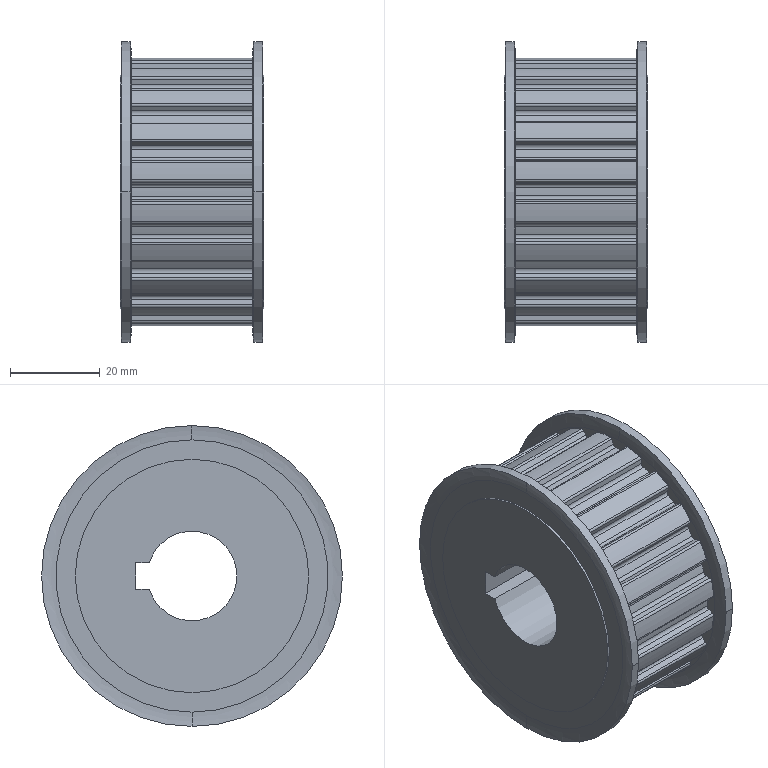Part | SolidWorks | features ICE 1, MBimport 1 | 1 solid | 187 faces | box 32 x 67 x 67 mm | volume 77303 mm3 | cylinder 130 | plane 49 | torus 8 | commonest cylinder face diameters 1.06 x40 1.72 x40 55.62 x20 59.88 x20 52 x4 67 x4